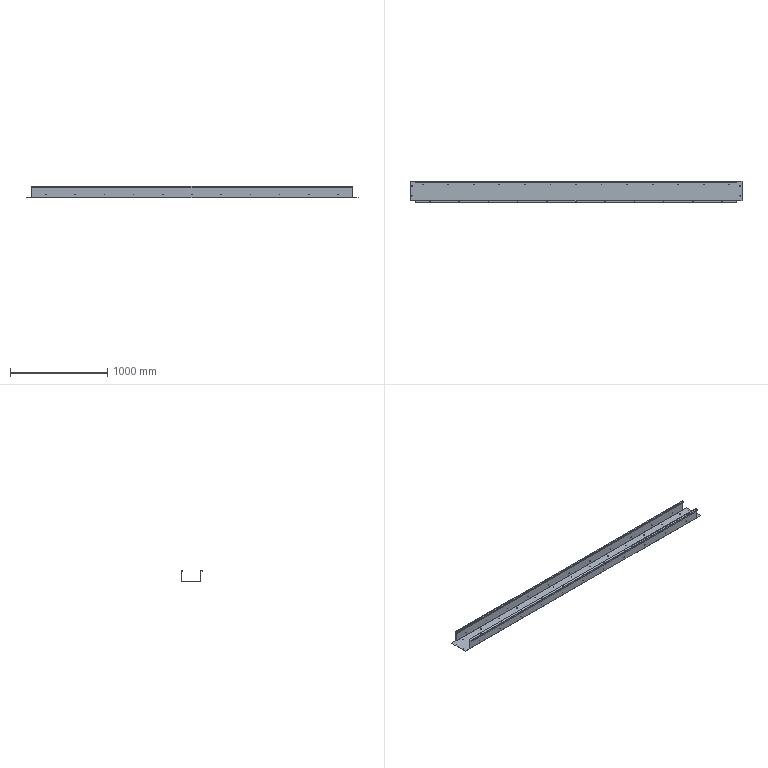Part | STEP file | TS-S24 | 1 solid | 214 faces | box 3411 x 225 x 122 mm | volume 3346088 mm3 | cylinder 134 | plane 80 | commonest cylinder face diameters 5.4 x66 7 x30 8.8 x26 0.4 x6 4.4 x6